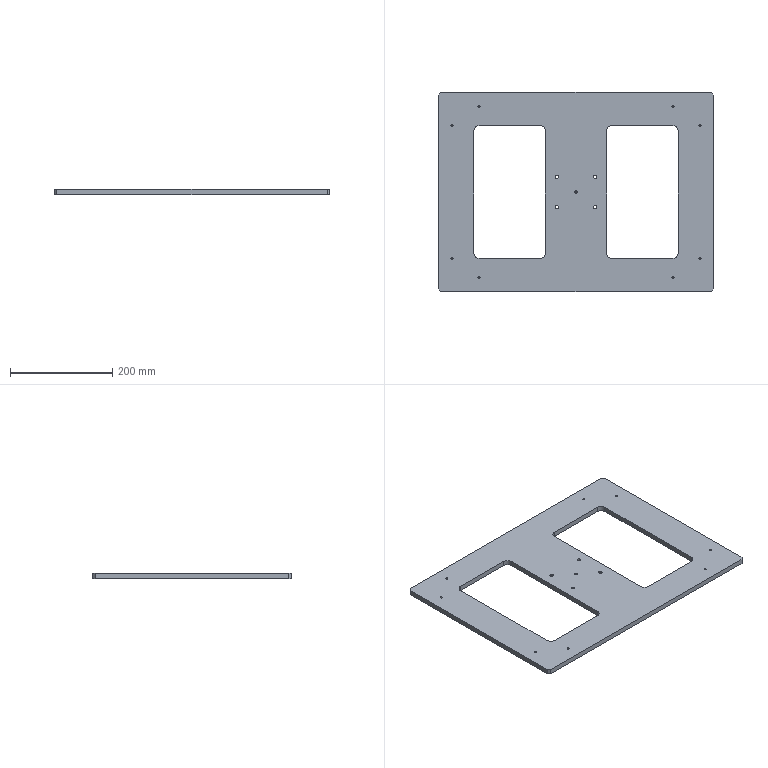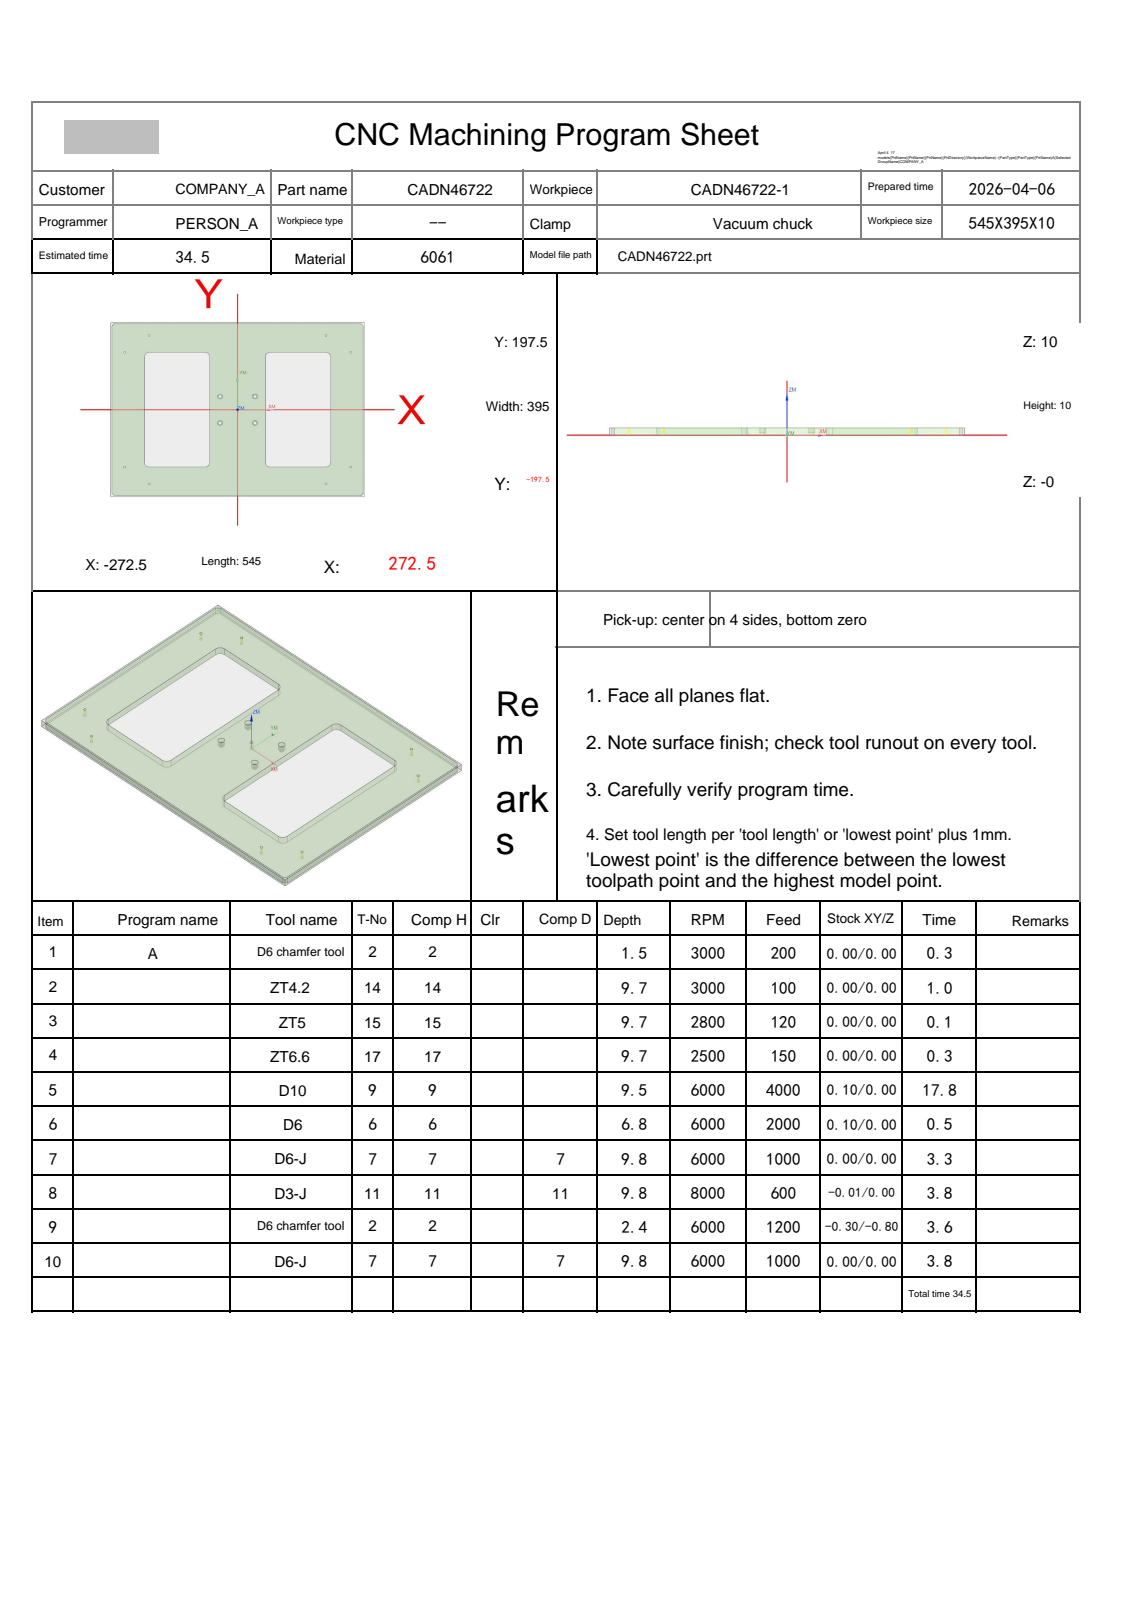NC program | NX | posted by the shop | part box 540 x 390 x 10 mm
Lines 3227 to 3473 of 3473:
N9 T02 M06
(D6 chamfer tool  D=6. R=0. H=02 ce=0.00 di=0.00)
G00 G90 G54 X.25 Y-197.128 M03 S6000
G43 H02 Z30.
M08
Z12.099
G01 Z8.5 F1200.
G03 X.33 Y-196.828 I-.52 J.3
X.03 Y-196.308 I-.6 J0.0
G01 X0.0 Y-196.3
X-265.
X-265.254 Y-196.275
X-265.497 Y-196.201
X-265.722 Y-196.081
X-265.919 Y-195.919
X-270.919 Y-190.919
X-271.081 Y-190.722
X-271.201 Y-190.497
X-271.275 Y-190.254
X-271.3 Y-190.
Y190.
X-271.275 Y190.254
X-271.201 Y190.497
X-271.081 Y190.722
X-270.919 Y190.919
X-265.919 Y195.919
X-265.722 Y196.081
X-265.497 Y196.201
X-265.254 Y196.275
X-265. Y196.3
X265.
X265.254 Y196.275
X265.497 Y196.201
X265.722 Y196.081
X265.919 Y195.919
X270.919 Y190.919
X271.081 Y190.722
X271.201 Y190.497
X271.275 Y190.254
X271.3 Y190.
Y-190.
X271.275 Y-190.254
X271.201 Y-190.497
X271.081 Y-190.722
X270.919 Y-190.919
X265.919 Y-195.919
X265.722 Y-196.081
X265.497 Y-196.201
X265.254 Y-196.275
X265. Y-196.3
X0.0
X-.03 Y-196.308
G03 X-.33 Y-196.828 I.3 J-.52
X-.25 Y-197.128 I.6 J0.0
G01 Z12.099
G00 Z30.
X-62.128 Y-.25
Z12.099
G01 Z8.5
G03 X-61.828 Y-.33 I.3 J.52
X-61.308 Y-.03 I0.0 J.6
G01 X-61.3 Y0.0
Y120.
G03 X-70. Y128.7 I-8.7 J0.0
G01 X-190.
G03 X-198.7 Y120. I0.0 J-8.7
G01 Y-120.
G03 X-190. Y-128.7 I8.7 J0.0
G01 X-70.
G03 X-61.3 Y-120. I0.0 J8.7
G01 Y0.0
X-61.308 Y.03
G03 X-61.828 Y.33 I-.52 J-.3
X-62.128 Y.25 I0.0 J-.6
G01 Z12.099
G00 Z30.
X62.128
Z12.099
G01 Z8.5
G03 X61.828 Y.33 I-.3 J-.52
X61.308 Y.03 I0.0 J-.6
G01 X61.3 Y0.0
Y-120.
G03 X70. Y-128.7 I8.7 J0.0
G01 X190.
G03 X198.7 Y-120. I0.0 J8.7
G01 Y120.
G03 X190. Y128.7 I-8.7 J0.0
G01 X70.
G03 X61.3 Y120. I0.0 J-8.7
G01 Y0.0
X61.308 Y-.03
G03 X61.828 Y-.33 I.52 J.3
X62.128 Y-.25 I0.0 J.6
G01 Z12.099
G00 Z30.
G00 G90 X190. Y-168. M03 S5000
Z30.
G98 G81 X190. Y-168. Z7.633 R13. F150.
X243. Y-130.
Y130.
X190. Y168.
X-190.
X-243. Y130.
Y-130.
X-190. Y-168.
G80
G00 Z30.
G00 G90 X.032 Y.095 M03 S6000
Z30.
Z8.9
G01 Z8.4 F600.
X.041 Y.123
G03 X-.381 Y.183 I-.423 J-1.439
X-1.1 Y0.0 I0.0 J-1.5
X0.0 Y-1.1 I1.1 J0.0
X1.1 Y0.0 I0.0 J1.1
X0.0 Y1.1 I-1.1 J0.0
X-1.1 Y0.0 I0.0 J-1.1
X-.381 Y-.183 I.719 J1.317
X.041 Y-.123 I0.0 J1.5
G01 X.032 Y-.095
Z8.9
G00 Z30.
G00 G90 X-38.221 Y-27.295 M03 S6000
Z30.
Z8.5
G01 Z8. F600.
X-38.3 Y-27.
G03 X-41.3 Y-30. I0.0 J-3.
X-37.5 Y-33.8 I3.8 J0.0
X-33.7 Y-30. I0.0 J3.8
X-37.5 Y-26.2 I-3.8 J0.0
X-41.3 Y-30. I0.0 J-3.8
X-38.3 Y-33. I3. J0.0
G01 X-38.221 Y-32.705
Z8.5
G00 Z30.
Y32.705
Z8.5
G01 Z8.
X-38.3 Y33.
G03 X-41.3 Y30. I0.0 J-3.
X-37.5 Y26.2 I3.8 J0.0
X-33.7 Y30. I0.0 J3.8
X-37.5 Y33.8 I-3.8 J0.0
X-41.3 Y30. I0.0 J-3.8
X-38.3 Y27. I3. J0.0
G01 X-38.221 Y27.295
Z8.5
G00 Z30.
X36.779 Y32.705
Z8.5
G01 Z8.
X36.7 Y33.
G03 X33.7 Y30. I0.0 J-3.
X37.5 Y26.2 I3.8 J0.0
X41.3 Y30. I0.0 J3.8
X37.5 Y33.8 I-3.8 J0.0
X33.7 Y30. I0.0 J-3.8
X36.7 Y27. I3. J0.0
G01 X36.779 Y27.295
Z8.5
G00 Z30.
Y-27.295
Z8.5
G01 Z8.
X36.7 Y-27.
G03 X33.7 Y-30. I0.0 J-3.
X37.5 Y-33.8 I3.8 J0.0
X41.3 Y-30. I0.0 J3.8
X37.5 Y-26.2 I-3.8 J0.0
X33.7 Y-30. I0.0 J-3.8
X36.7 Y-33. I3. J0.0
G01 X36.779 Y-32.705
Z8.5
G00 Z30.
G91 G28 Z0.0
M05
M09
G91 G28 Z0.0
M01
N10 T07 M06
(D6-J  D=6. R=0. H=07 ce=0.00 di=0.00)
G00 G90 G54 X266.017 Y-199.073 M03 S6000
G43 H07 Z30.
M08
Z1.
G01 Z.5 F1000.
G41 D07
X265.992 Y-198.875
G03 X265. Y-198. I-.992 J-.125
G01 X-265.
G02 X-267.121 Y-197.121 I0.0 J3.
G01 X-272.121 Y-192.121
G02 X-273. Y-190. I2.121 J2.121
G01 Y190.
G02 X-272.121 Y192.121 I3. J0.0
G01 X-267.121 Y197.121
G02 X-265. Y198. I2.121 J-2.121
G01 X265.
G02 X267.121 Y197.121 I0.0 J-3.
G01 X272.121 Y192.121
G02 X273. Y190. I-2.121 J-2.121
G01 Y-190.
G02 X272.121 Y-192.121 I-3. J0.0
G01 X267.121 Y-197.121
G02 X265. Y-198. I-2.121 J2.121
G01 X264.5
G03 X263.5 Y-199. I0.0 J-1.
G01 G40 Y-199.2
Z1.
G00 Z30.
G00 G90 X266.005 Y-198.974 M03 S6000
Z30.
Z.7
G01 Z.2 F1000.
G41 D07
X265.992 Y-198.875
G03 X265. Y-198. I-.992 J-.125
G01 X-265.
G02 X-267.121 Y-197.121 I0.0 J3.
G01 X-272.121 Y-192.121
G02 X-273. Y-190. I2.121 J2.121
G01 Y190.
G02 X-272.121 Y192.121 I3. J0.0
G01 X-267.121 Y197.121
G02 X-265. Y198. I2.121 J-2.121
G01 X265.
G02 X267.121 Y197.121 I0.0 J-3.
G01 X272.121 Y192.121
G02 X273. Y190. I-2.121 J-2.121
G01 Y-190.
G02 X272.121 Y-192.121 I-3. J0.0
G01 X267.121 Y-197.121
G02 X265. Y-198. I-2.121 J2.121
G01 X264.5
G03 X263.5 Y-199. I0.0 J-1.
G01 G40 Y-199.1
Z.7
G00 Z30.
M05
M09
G91 G28 Z0.0
G91 G28 Y0.0
M30
%